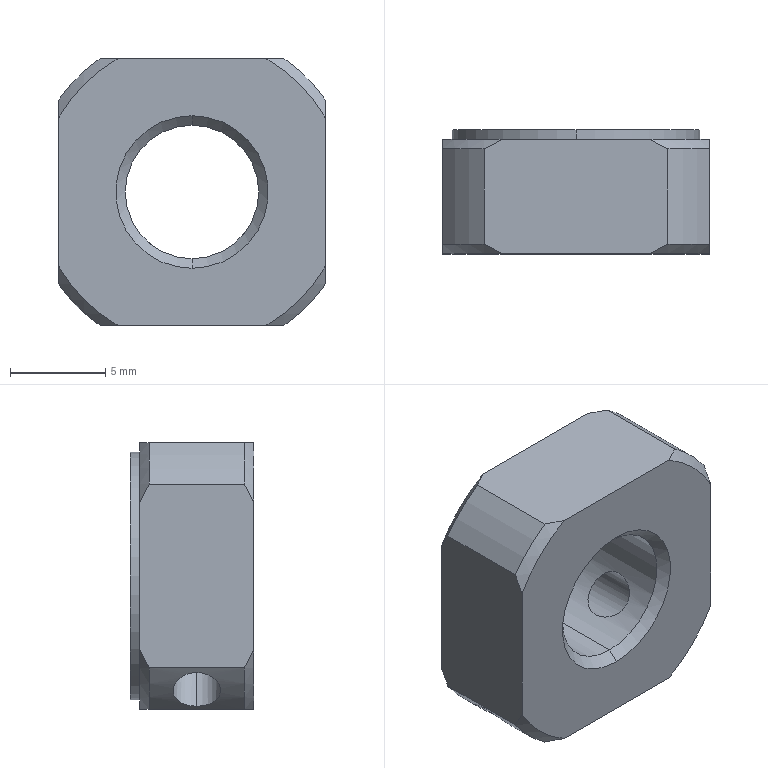Part | SolidWorks | features Chamfer 2, HoleWzd 2, ICE 2, CirPattern 1, Extrusion 1 | 1 solid | 31 faces | box 14 x 6.5 x 14 mm | volume 883.515 mm3 | cylinder 12 | cone 12 | plane 7 | commonest cylinder face diameters 2.5 x4 17 x4 7 x2 13 x2
STEP:
#1=CARTESIAN_POINT('',(-6.829,-3.,-5.061));
#2=VERTEX_POINT('',#1);
#3=CARTESIAN_POINT('',(-5.061,-3.,-6.829));
#4=VERTEX_POINT('',#3);
#5=CARTESIAN_POINT('',(-6.829,-3.,-5.061));
#6=CARTESIAN_POINT('',(-6.829,-3.163,-5.061));
#7=CARTESIAN_POINT('',(-6.809,-3.328,-5.088));
#8=CARTESIAN_POINT('',(-6.733,-3.629,-5.188));
#9=CARTESIAN_POINT('',(-6.676,-3.768,-5.262));
#10=CARTESIAN_POINT('',(-6.567,-3.941,-5.397));
#11=CARTESIAN_POINT('',(-6.526,-3.994,-5.447));
#12=CARTESIAN_POINT('',(-6.438,-4.084,-5.551));
#13=CARTESIAN_POINT('',(-6.391,-4.123,-5.605));
#14=CARTESIAN_POINT('',(-6.239,-4.217,-5.775));
#15=CARTESIAN_POINT('',(-6.128,-4.25,-5.893));
#16=CARTESIAN_POINT('',(-5.894,-4.25,-6.127));
#17=CARTESIAN_POINT('',(-5.776,-4.218,-6.238));
#18=CARTESIAN_POINT('',(-5.55,-4.092,-6.44));
#19=CARTESIAN_POINT('',(-5.443,-3.999,-6.53));
#20=CARTESIAN_POINT('',(-5.263,-3.769,-6.675));
#21=CARTESIAN_POINT('',(-5.189,-3.63,-6.733));
#22=CARTESIAN_POINT('',(-5.088,-3.33,-6.809));
#23=CARTESIAN_POINT('',(-5.061,-3.165,-6.829));
#24=CARTESIAN_POINT('',(-5.061,-3.,-6.829));
#25=B_SPLINE_CURVE_WITH_KNOTS('',3,(#5,#6,#7,#8,#9,#10,#11,#12,#13,#14,#15,#16,#17,#18,#19,#20,#21,#22,#23,#24),.UNSPECIFIED.,.F.,.F.,(4,2,2,2,2,2,2,2,2,4),(0.003913,0.004402,0.004891,0.005136,0.005381,0.00587,0.006359,0.006848,0.007337,0.007826),.UNSPECIFIED.);
#26=EDGE_CURVE('',#2,#4,#25,.T.);
#27=ORIENTED_EDGE('',*,*,#26,.F.);
#28=CARTESIAN_POINT('',(-3.196,-3.,-1.428));
#29=VERTEX_POINT('',#28);
#30=CARTESIAN_POINT('',(-0.8839,-3.,0.8839));
#31=DIRECTION('',(0.7071,0.,0.7071));
#32=VECTOR('',#31,1000.);
#33=LINE('',#30,#32);
#34=EDGE_CURVE('',#2,#29,#33,.T.);
#35=ORIENTED_EDGE('',*,*,#34,.T.);
#36=CARTESIAN_POINT('',(-1.428,-3.,-3.196));
#37=VERTEX_POINT('',#36);
#38=CARTESIAN_POINT('',(-1.428,-3.,-3.196));
#39=CARTESIAN_POINT('',(-1.428,-3.167,-3.196));
#40=CARTESIAN_POINT('',(-1.461,-3.33,-3.181));
#41=CARTESIAN_POINT('',(-1.581,-3.632,-3.123));
#42=CARTESIAN_POINT('',(-1.668,-3.77,-3.079));
#43=CARTESIAN_POINT('',(-1.872,-3.998,-2.96));
#44=CARTESIAN_POINT('',(-1.99,-4.091,-2.883));
#45=CARTESIAN_POINT('',(-2.232,-4.216,-2.7));
#46=CARTESIAN_POINT('',(-2.358,-4.25,-2.592));
#47=CARTESIAN_POINT('',(-2.533,-4.25,-2.417));
#48=CARTESIAN_POINT('',(-2.59,-4.242,-2.356));
#49=CARTESIAN_POINT('',(-2.695,-4.209,-2.234));
#50=CARTESIAN_POINT('',(-2.745,-4.186,-2.173));
#51=CARTESIAN_POINT('',(-2.884,-4.09,-1.989));
#52=CARTESIAN_POINT('',(-2.96,-3.998,-1.871));
#53=CARTESIAN_POINT('',(-3.05,-3.826,-1.718));
#54=CARTESIAN_POINT('',(-3.076,-3.763,-1.671));
#55=CARTESIAN_POINT('',(-3.12,-3.628,-1.587));
#56=CARTESIAN_POINT('',(-3.138,-3.555,-1.55));
#57=CARTESIAN_POINT('',(-3.181,-3.33,-1.461));
#58=CARTESIAN_POINT('',(-3.196,-3.164,-1.428));
#59=CARTESIAN_POINT('',(-3.196,-3.,-1.428));
#60=B_SPLINE_CURVE_WITH_KNOTS('',3,(#38,#39,#40,#41,#42,#43,#44,#45,#46,#47,#48,#49,#50,#51,#52,#53,#54,#55,#56,#57,#58,#59),.UNSPECIFIED.,.F.,.F.,(4,2,2,2,2,2,2,2,2,2,4),(0.,0.0004926,0.0009852,0.001478,0.00197,0.002217,0.002463,0.002956,0.003202,0.003448,0.003941),.UNSPECIFIED.);
#61=EDGE_CURVE('',#37,#29,#60,.T.);
#62=ORIENTED_EDGE('',*,*,#61,.F.);
#63=CARTESIAN_POINT('',(0.8839,-3.,-0.8839));
#64=DIRECTION('',(0.7071,0.,0.7071));
#65=VECTOR('',#64,1000.);
#66=LINE('',#63,#65);
#67=EDGE_CURVE('',#4,#37,#66,.T.);
#68=ORIENTED_EDGE('',*,*,#67,.F.);
#69=EDGE_LOOP('',(#27,#35,#62,#68));
#70=FACE_OUTER_BOUND('',#69,.T.);
#71=CARTESIAN_POINT('',(0.,-3.,0.));
#72=DIRECTION('',(0.7071,0.,0.7071));
#73=DIRECTION('',(0.7071,0.,-0.7071));
#74=AXIS2_PLACEMENT_3D('',#71,#72,#73);
#75=CYLINDRICAL_SURFACE('',#74,1.25);
#76=ADVANCED_FACE('',(#70),#75,.F.);
#77=CARTESIAN_POINT('',(0.,0.,-3.5));
#78=VERTEX_POINT('',#77);
#79=CARTESIAN_POINT('',(0.,0.,3.5));
#80=VERTEX_POINT('',#79);
#81=CARTESIAN_POINT('',(0.,0.,0.));
#82=DIRECTION('',(0.,1.,0.));
#83=DIRECTION('',(0.,0.,1.));
#84=AXIS2_PLACEMENT_3D('',#81,#82,#83);
#85=CIRCLE('',#84,3.5);
#86=EDGE_CURVE('',#78,#80,#85,.T.);
#87=ORIENTED_EDGE('',*,*,#86,.F.);
#88=CARTESIAN_POINT('',(0.,0.5,-4.));
#89=VERTEX_POINT('',#88);
#90=CARTESIAN_POINT('',(0.,0.,-3.5));
#91=DIRECTION('',(0.,0.7071,-0.7071));
#92=VECTOR('',#91,1000.);
#93=LINE('',#90,#92);
#94=EDGE_CURVE('',#78,#89,#93,.T.);
#95=ORIENTED_EDGE('',*,*,#94,.T.);
#96=CARTESIAN_POINT('',(0.,0.5,4.));
#97=VERTEX_POINT('',#96);
#98=CARTESIAN_POINT('',(0.,0.5,0.));
#99=DIRECTION('',(0.,-1.,0.));
#100=DIRECTION('',(0.,0.,1.));
#101=AXIS2_PLACEMENT_3D('',#98,#99,#100);
#102=CIRCLE('',#101,4.);
#103=EDGE_CURVE('',#97,#89,#102,.T.);
#104=ORIENTED_EDGE('',*,*,#103,.F.);
#105=CARTESIAN_POINT('',(0.,0.,3.5));
#106=DIRECTION('',(0.,0.7071,0.7071));
#107=VECTOR('',#106,1000.);
#108=LINE('',#105,#107);
#109=EDGE_CURVE('',#80,#97,#108,.T.);
#110=ORIENTED_EDGE('',*,*,#109,.F.);
#111=EDGE_LOOP('',(#87,#95,#104,#110));
#112=FACE_OUTER_BOUND('',#111,.T.);
#113=CARTESIAN_POINT('',(0.,0.,0.));
#114=DIRECTION('',(0.,1.,0.));
#115=DIRECTION('',(0.,0.,1.));
#116=AXIS2_PLACEMENT_3D('',#113,#114,#115);
#117=CONICAL_SURFACE('',#116,3.5,0.7854);
#118=ADVANCED_FACE('',(#112),#117,.F.);
#119=CARTESIAN_POINT('',(0.,-5.5,3.5));
#120=VERTEX_POINT('',#119);
#121=CARTESIAN_POINT('',(0.,-5.5,-3.5));
#122=VERTEX_POINT('',#121);
#123=CARTESIAN_POINT('',(0.,-5.5,0.));
#124=DIRECTION('',(0.,-1.,0.));
#125=DIRECTION('',(0.,0.,-1.));
#126=AXIS2_PLACEMENT_3D('',#123,#124,#125);
#127=CIRCLE('',#126,3.5);
#128=EDGE_CURVE('',#120,#122,#127,.T.);
#129=ORIENTED_EDGE('',*,*,#128,.F.);
#130=CARTESIAN_POINT('',(0.,-6.,4.));
#131=VERTEX_POINT('',#130);
#132=CARTESIAN_POINT('',(0.,-5.5,3.5));
#133=DIRECTION('',(0.,-0.7071,0.7071));
#134=VECTOR('',#133,1000.);
#135=LINE('',#132,#134);
#136=EDGE_CURVE('',#120,#131,#135,.T.);
#137=ORIENTED_EDGE('',*,*,#136,.T.);
#138=CARTESIAN_POINT('',(0.,-6.,-4.));
#139=VERTEX_POINT('',#138);
#140=CARTESIAN_POINT('',(0.,-6.,0.));
#141=DIRECTION('',(0.,1.,0.));
#142=DIRECTION('',(0.,0.,-1.));
#143=AXIS2_PLACEMENT_3D('',#140,#141,#142);
#144=CIRCLE('',#143,4.);
#145=EDGE_CURVE('',#139,#131,#144,.T.);
#146=ORIENTED_EDGE('',*,*,#145,.F.);
#147=CARTESIAN_POINT('',(0.,-5.5,-3.5));
#148=DIRECTION('',(0.,-0.7071,-0.7071));
#149=VECTOR('',#148,1000.);
#150=LINE('',#147,#149);
#151=EDGE_CURVE('',#122,#139,#150,.T.);
#152=ORIENTED_EDGE('',*,*,#151,.F.);
#153=EDGE_LOOP('',(#129,#137,#146,#152));
#154=FACE_OUTER_BOUND('',#153,.T.);
#155=CARTESIAN_POINT('',(0.,-5.5,0.));
#156=DIRECTION('',(0.,-1.,0.));
#157=DIRECTION('',(0.,0.,-1.));
#158=AXIS2_PLACEMENT_3D('',#155,#156,#157);
#159=CONICAL_SURFACE('',#158,3.5,0.7854);
#160=ADVANCED_FACE('',(#154),#159,.F.);
#161=CARTESIAN_POINT('',(5.061,-3.,-6.829));
#162=VERTEX_POINT('',#161);
#163=CARTESIAN_POINT('',(6.829,-3.,-5.061));
#164=VERTEX_POINT('',#163);
#165=CARTESIAN_POINT('',(5.061,-3.,-6.829));
#166=CARTESIAN_POINT('',(5.061,-3.163,-6.829));
#167=CARTESIAN_POINT('',(5.088,-3.328,-6.809));
#168=CARTESIAN_POINT('',(5.188,-3.629,-6.733));
#169=CARTESIAN_POINT('',(5.262,-3.768,-6.676));
#170=CARTESIAN_POINT('',(5.397,-3.941,-6.567));
#171=CARTESIAN_POINT('',(5.447,-3.994,-6.526));
#172=CARTESIAN_POINT('',(5.551,-4.084,-6.438));
#173=CARTESIAN_POINT('',(5.605,-4.123,-6.391));
#174=CARTESIAN_POINT('',(5.775,-4.217,-6.239));
#175=CARTESIAN_POINT('',(5.893,-4.25,-6.128));
#176=CARTESIAN_POINT('',(6.127,-4.25,-5.894));
#177=CARTESIAN_POINT('',(6.238,-4.218,-5.776));
#178=CARTESIAN_POINT('',(6.44,-4.092,-5.55));
#179=CARTESIAN_POINT('',(6.53,-3.999,-5.443));
#180=CARTESIAN_POINT('',(6.675,-3.769,-5.263));
#181=CARTESIAN_POINT('',(6.733,-3.63,-5.189));
#182=CARTESIAN_POINT('',(6.809,-3.33,-5.088));
#183=CARTESIAN_POINT('',(6.829,-3.165,-5.061));
#184=CARTESIAN_POINT('',(6.829,-3.,-5.061));
#185=B_SPLINE_CURVE_WITH_KNOTS('',3,(#165,#166,#167,#168,#169,#170,#171,#172,#173,#174,#175,#176,#177,#178,#179,#180,#181,#182,#183,#184),.UNSPECIFIED.,.F.,.F.,(4,2,2,2,2,2,2,2,2,4),(0.003913,0.004402,0.004891,0.005136,0.005381,0.00587,0.006359,0.006848,0.007337,0.007826),.UNSPECIFIED.);
#186=EDGE_CURVE('',#162,#164,#185,.T.);
#187=ORIENTED_EDGE('',*,*,#186,.F.);
#188=CARTESIAN_POINT('',(1.428,-3.,-3.196));
#189=VERTEX_POINT('',#188);
#190=CARTESIAN_POINT('',(-0.8839,-3.,-0.8839));
#191=DIRECTION('',(-0.7071,0.,0.7071));
#192=VECTOR('',#191,1000.);
#193=LINE('',#190,#192);
#194=EDGE_CURVE('',#162,#189,#193,.T.);
#195=ORIENTED_EDGE('',*,*,#194,.T.);
#196=CARTESIAN_POINT('',(3.196,-3.,-1.428));
#197=VERTEX_POINT('',#196);
#198=CARTESIAN_POINT('',(3.196,-3.,-1.428));
#199=CARTESIAN_POINT('',(3.196,-3.167,-1.428));
#200=CARTESIAN_POINT('',(3.181,-3.33,-1.461));
#201=CARTESIAN_POINT('',(3.123,-3.632,-1.581));
#202=CARTESIAN_POINT('',(3.079,-3.77,-1.668));
#203=CARTESIAN_POINT('',(2.96,-3.998,-1.872));
#204=CARTESIAN_POINT('',(2.883,-4.091,-1.99));
#205=CARTESIAN_POINT('',(2.7,-4.216,-2.232));
#206=CARTESIAN_POINT('',(2.592,-4.25,-2.358));
#207=CARTESIAN_POINT('',(2.417,-4.25,-2.533));
#208=CARTESIAN_POINT('',(2.356,-4.242,-2.59));
#209=CARTESIAN_POINT('',(2.234,-4.209,-2.695));
#210=CARTESIAN_POINT('',(2.173,-4.186,-2.745));
#211=CARTESIAN_POINT('',(1.989,-4.09,-2.884));
#212=CARTESIAN_POINT('',(1.871,-3.998,-2.96));
#213=CARTESIAN_POINT('',(1.718,-3.826,-3.05));
#214=CARTESIAN_POINT('',(1.671,-3.763,-3.076));
#215=CARTESIAN_POINT('',(1.587,-3.628,-3.12));
#216=CARTESIAN_POINT('',(1.55,-3.555,-3.138));
#217=CARTESIAN_POINT('',(1.461,-3.33,-3.181));
#218=CARTESIAN_POINT('',(1.428,-3.164,-3.196));
#219=CARTESIAN_POINT('',(1.428,-3.,-3.196));
#220=B_SPLINE_CURVE_WITH_KNOTS('',3,(#198,#199,#200,#201,#202,#203,#204,#205,#206,#207,#208,#209,#210,#211,#212,#213,#214,#215,#216,#217,#218,#219),.UNSPECIFIED.,.F.,.F.,(4,2,2,2,2,2,2,2,2,2,4),(0.,0.0004926,0.0009852,0.001478,0.00197,0.002217,0.002463,0.002956,0.003202,0.003448,0.003941),.UNSPECIFIED.);
#221=EDGE_CURVE('',#197,#189,#220,.T.);
#222=ORIENTED_EDGE('',*,*,#221,.F.);
#223=CARTESIAN_POINT('',(0.8839,-3.,0.8839));
#224=DIRECTION('',(-0.7071,0.,0.7071));
#225=VECTOR('',#224,1000.);
#226=LINE('',#223,#225);
#227=EDGE_CURVE('',#164,#197,#226,.T.);
#228=ORIENTED_EDGE('',*,*,#227,.F.);
#229=EDGE_LOOP('',(#187,#195,#222,#228));
#230=FACE_OUTER_BOUND('',#229,.T.);
#231=CARTESIAN_POINT('',(0.,-3.,0.));
#232=DIRECTION('',(-0.7071,0.,0.7071));
#233=DIRECTION('',(0.7071,0.,0.7071));
#234=AXIS2_PLACEMENT_3D('',#231,#232,#233);
#235=CYLINDRICAL_SURFACE('',#234,1.25);
#236=ADVANCED_FACE('',(#230),#235,.F.);
#237=ORIENTED_EDGE('',*,*,#61,.T.);
#238=CARTESIAN_POINT('',(-3.196,-3.,-1.428));
#239=CARTESIAN_POINT('',(-3.196,-2.836,-1.428));
#240=CARTESIAN_POINT('',(-3.181,-2.67,-1.461));
#241=CARTESIAN_POINT('',(-3.124,-2.369,-1.58));
#242=CARTESIAN_POINT('',(-3.08,-2.232,-1.667));
#243=CARTESIAN_POINT('',(-2.959,-2.,-1.873));
#244=CARTESIAN_POINT('',(-2.883,-1.909,-1.99));
#245=CARTESIAN_POINT('',(-2.745,-1.814,-2.173));
#246=CARTESIAN_POINT('',(-2.695,-1.791,-2.234));
#247=CARTESIAN_POINT('',(-2.59,-1.758,-2.356));
#248=CARTESIAN_POINT('',(-2.533,-1.75,-2.417));
#249=CARTESIAN_POINT('',(-2.358,-1.75,-2.592));
#250=CARTESIAN_POINT('',(-2.232,-1.784,-2.7));
#251=CARTESIAN_POINT('',(-1.99,-1.909,-2.883));
#252=CARTESIAN_POINT('',(-1.871,-2.002,-2.96));
#253=CARTESIAN_POINT('',(-1.667,-2.231,-3.08));
#254=CARTESIAN_POINT('',(-1.581,-2.368,-3.123));
#255=CARTESIAN_POINT('',(-1.46,-2.671,-3.181));
#256=CARTESIAN_POINT('',(-1.428,-2.833,-3.196));
#257=CARTESIAN_POINT('',(-1.428,-3.,-3.196));
#258=B_SPLINE_CURVE_WITH_KNOTS('',3,(#238,#239,#240,#241,#242,#243,#244,#245,#246,#247,#248,#249,#250,#251,#252,#253,#254,#255,#256,#257),.UNSPECIFIED.,.F.,.F.,(4,2,2,2,2,2,2,2,2,4),(0.003941,0.004433,0.004926,0.005418,0.005664,0.005911,0.006403,0.006896,0.007388,0.007881),.UNSPECIFIED.);
#259=EDGE_CURVE('',#29,#37,#258,.T.);
#260=ORIENTED_EDGE('',*,*,#259,.T.);
#261=EDGE_LOOP('',(#237,#260));
#262=FACE_BOUND('',#261,.T.);
#263=ORIENTED_EDGE('',*,*,#128,.T.);
#264=CARTESIAN_POINT('',(0.,0.5,-3.5));
#265=DIRECTION('',(0.,1.,0.));
#266=VECTOR('',#265,1000.);
#267=LINE('',#264,#266);
#268=EDGE_CURVE('',#122,#78,#267,.T.);
#269=ORIENTED_EDGE('',*,*,#268,.T.);
#270=ORIENTED_EDGE('',*,*,#86,.T.);
#271=CARTESIAN_POINT('',(0.,0.5,3.5));
#272=DIRECTION('',(0.,1.,0.));
#273=VECTOR('',#272,1000.);
#274=LINE('',#271,#273);
#275=EDGE_CURVE('',#120,#80,#274,.T.);
#276=ORIENTED_EDGE('',*,*,#275,.F.);
#277=EDGE_LOOP('',(#263,#269,#270,#276));
#278=FACE_OUTER_BOUND('',#277,.T.);
#279=CARTESIAN_POINT('',(0.,0.5,0.));
#280=DIRECTION('',(0.,1.,0.));
#281=DIRECTION('',(0.,0.,1.));
#282=AXIS2_PLACEMENT_3D('',#279,#280,#281);
#283=CYLINDRICAL_SURFACE('',#282,3.5);
#284=ADVANCED_FACE('',(#262,#278),#283,.F.);
#285=CARTESIAN_POINT('',(0.,0.5,6.5));
#286=VERTEX_POINT('',#285);
#287=CARTESIAN_POINT('',(0.,0.5,-6.5));
#288=VERTEX_POINT('',#287);
#289=CARTESIAN_POINT('',(0.,0.5,0.));
#290=DIRECTION('',(0.,1.,0.));
#291=DIRECTION('',(0.,0.,1.));
#292=AXIS2_PLACEMENT_3D('',#289,#290,#291);
#293=CIRCLE('',#292,6.5);
#294=EDGE_CURVE('',#286,#288,#293,.T.);
#295=ORIENTED_EDGE('',*,*,#294,.F.);
#296=CARTESIAN_POINT('',(0.,0.,6.5));
#297=VERTEX_POINT('',#296);
#298=CARTESIAN_POINT('',(0.,0.5,6.5));
#299=DIRECTION('',(0.,-1.,0.));
#300=VECTOR('',#299,1000.);
#301=LINE('',#298,#300);
#302=EDGE_CURVE('',#286,#297,#301,.T.);
#303=ORIENTED_EDGE('',*,*,#302,.T.);
#304=CARTESIAN_POINT('',(0.,0.,-6.5));
#305=VERTEX_POINT('',#304);
#306=CARTESIAN_POINT('',(0.,0.,0.));
#307=DIRECTION('',(0.,-1.,0.));
#308=DIRECTION('',(0.,0.,-1.));
#309=AXIS2_PLACEMENT_3D('',#306,#307,#308);
#310=CIRCLE('',#309,6.5);
#311=EDGE_CURVE('',#305,#297,#310,.T.);
#312=ORIENTED_EDGE('',*,*,#311,.F.);
#313=CARTESIAN_POINT('',(0.,0.5,-6.5));
#314=DIRECTION('',(0.,-1.,0.));
#315=VECTOR('',#314,1000.);
#316=LINE('',#313,#315);
#317=EDGE_CURVE('',#288,#305,#316,.T.);
#318=ORIENTED_EDGE('',*,*,#317,.F.);
#319=EDGE_LOOP('',(#295,#303,#312,#318));
#320=FACE_OUTER_BOUND('',#319,.T.);
#321=CARTESIAN_POINT('',(0.,0.5,0.));
#322=DIRECTION('',(0.,-1.,0.));
#323=DIRECTION('',(0.,0.,-1.));
#324=AXIS2_PLACEMENT_3D('',#321,#322,#323);
#325=CYLINDRICAL_SURFACE('',#324,6.5);
#326=ADVANCED_FACE('',(#320),#325,.T.);
#327=CARTESIAN_POINT('',(-7.,-5.5,4.822));
#328=VERTEX_POINT('',#327);
#329=CARTESIAN_POINT('',(-4.822,-5.5,7.));
#330=VERTEX_POINT('',#329);
#331=CARTESIAN_POINT('',(0.,-5.5,0.));
#332=DIRECTION('',(0.,1.,0.));
#333=DIRECTION('',(0.,0.,-1.));
#334=AXIS2_PLACEMENT_3D('',#331,#332,#333);
#335=CIRCLE('',#334,8.5);
#336=EDGE_CURVE('',#328,#330,#335,.T.);
#337=ORIENTED_EDGE('',*,*,#336,.T.);
#338=CARTESIAN_POINT('',(-4.822,-0.5,7.));
#339=VERTEX_POINT('',#338);
#340=CARTESIAN_POINT('',(-4.822,-6.,7.));
#341=DIRECTION('',(0.,1.,0.));
#342=VECTOR('',#341,1000.);
#343=LINE('',#340,#342);
#344=EDGE_CURVE('',#330,#339,#343,.T.);
#345=ORIENTED_EDGE('',*,*,#344,.T.);
#346=CARTESIAN_POINT('',(-7.,-0.5,4.822));
#347=VERTEX_POINT('',#346);
#348=CARTESIAN_POINT('',(0.,-0.5,0.));
#349=DIRECTION('',(0.,-1.,0.));
#350=DIRECTION('',(0.,0.,-1.));
#351=AXIS2_PLACEMENT_3D('',#348,#349,#350);
#352=CIRCLE('',#351,8.5);
#353=EDGE_CURVE('',#339,#347,#352,.T.);
#354=ORIENTED_EDGE('',*,*,#353,.T.);
#355=CARTESIAN_POINT('',(-7.,-6.,4.822));
#356=DIRECTION('',(0.,-1.,0.));
#357=VECTOR('',#356,1000.);
#358=LINE('',#355,#357);
#359=EDGE_CURVE('',#347,#328,#358,.T.);
#360=ORIENTED_EDGE('',*,*,#359,.T.);
#361=EDGE_LOOP('',(#337,#345,#354,#360));
#362=FACE_OUTER_BOUND('',#361,.T.);
#363=CARTESIAN_POINT('',(0.,-6.,0.));
#364=DIRECTION('',(0.,1.,0.));
#365=DIRECTION('',(0.,0.,1.));
#366=AXIS2_PLACEMENT_3D('',#363,#364,#365);
#367=CYLINDRICAL_SURFACE('',#366,8.5);
#368=ADVANCED_FACE('',(#362),#367,.T.);
#369=CARTESIAN_POINT('',(-3.873,-6.,7.));
#370=VERTEX_POINT('',#369);
#371=CARTESIAN_POINT('',(-4.822,-5.5,7.));
#372=CARTESIAN_POINT('',(-4.511,-5.676,7.));
#373=CARTESIAN_POINT('',(-4.195,-5.844,7.));
#374=CARTESIAN_POINT('',(-3.873,-6.,7.));
#375=B_SPLINE_CURVE_WITH_KNOTS('',3,(#371,#372,#373,#374),.UNSPECIFIED.,.F.,.F.,(4,4),(0.00829,0.009369),.UNSPECIFIED.);
#376=EDGE_CURVE('',#330,#370,#375,.T.);
#377=ORIENTED_EDGE('',*,*,#376,.F.);
#378=ORIENTED_EDGE('',*,*,#336,.F.);
#379=CARTESIAN_POINT('',(-7.,-6.,3.873));
#380=VERTEX_POINT('',#379);
#381=CARTESIAN_POINT('',(-7.,-6.,3.873));
#382=CARTESIAN_POINT('',(-7.,-5.844,4.195));
#383=CARTESIAN_POINT('',(-7.,-5.676,4.511));
#384=CARTESIAN_POINT('',(-7.,-5.5,4.822));
#385=B_SPLINE_CURVE_WITH_KNOTS('',3,(#381,#382,#383,#384),.UNSPECIFIED.,.F.,.F.,(4,4),(0.02473,0.02581),.UNSPECIFIED.);
#386=EDGE_CURVE('',#380,#328,#385,.T.);
#387=ORIENTED_EDGE('',*,*,#386,.F.);
#388=CARTESIAN_POINT('',(0.,-6.,0.));
#389=DIRECTION('',(0.,-1.,0.));
#390=DIRECTION('',(0.,0.,-1.));
#391=AXIS2_PLACEMENT_3D('',#388,#389,#390);
#392=CIRCLE('',#391,8.);
#393=EDGE_CURVE('',#370,#380,#392,.T.);
#394=ORIENTED_EDGE('',*,*,#393,.F.);
#395=EDGE_LOOP('',(#377,#378,#387,#394));
#396=FACE_OUTER_BOUND('',#395,.T.);
#397=CARTESIAN_POINT('',(0.,-6.,0.));
#398=DIRECTION('',(0.,1.,0.));
#399=DIRECTION('',(0.,0.,1.));
#400=AXIS2_PLACEMENT_3D('',#397,#398,#399);
#401=CONICAL_SURFACE('',#400,8.,0.7854);
#402=ADVANCED_FACE('',(#396),#401,.T.);
#403=CARTESIAN_POINT('',(4.822,-0.5,7.));
#404=VERTEX_POINT('',#403);
#405=CARTESIAN_POINT('',(3.873,0.,7.));
#406=VERTEX_POINT('',#405);
#407=CARTESIAN_POINT('',(4.822,-0.5,7.));
#408=CARTESIAN_POINT('',(4.511,-0.3235,7.));
#409=CARTESIAN_POINT('',(4.195,-0.1559,7.));
#410=CARTESIAN_POINT('',(3.873,0.,7.));
#411=B_SPLINE_CURVE_WITH_KNOTS('',3,(#407,#408,#409,#410),.UNSPECIFIED.,.F.,.F.,(4,4),(0.007915,0.008995),.UNSPECIFIED.);
#412=EDGE_CURVE('',#404,#406,#411,.T.);
#413=ORIENTED_EDGE('',*,*,#412,.F.);
#414=CARTESIAN_POINT('',(7.,-0.5,4.822));
#415=VERTEX_POINT('',#414);
#416=CARTESIAN_POINT('',(0.,-0.5,0.));
#417=DIRECTION('',(0.,-1.,0.));
#418=DIRECTION('',(0.,0.,-1.));
#419=AXIS2_PLACEMENT_3D('',#416,#417,#418);
#420=CIRCLE('',#419,8.5);
#421=EDGE_CURVE('',#415,#404,#420,.T.);
#422=ORIENTED_EDGE('',*,*,#421,.F.);
#423=CARTESIAN_POINT('',(7.,0.,3.873));
#424=VERTEX_POINT('',#423);
#425=CARTESIAN_POINT('',(7.,0.,3.873));
#426=CARTESIAN_POINT('',(7.,-0.1561,4.196));
#427=CARTESIAN_POINT('',(7.,-0.3238,4.511));
#428=CARTESIAN_POINT('',(7.,-0.5,4.822));
#429=B_SPLINE_CURVE_WITH_KNOTS('',3,(#425,#426,#427,#428),.UNSPECIFIED.,.F.,.F.,(4,4),(0.02391,0.025),.UNSPECIFIED.);
#430=EDGE_CURVE('',#424,#415,#429,.T.);
#431=ORIENTED_EDGE('',*,*,#430,.F.);
#432=CARTESIAN_POINT('',(0.,0.,0.));
#433=DIRECTION('',(0.,1.,0.));
#434=DIRECTION('',(0.,0.,-1.));
#435=AXIS2_PLACEMENT_3D('',#432,#433,#434);
#436=CIRCLE('',#435,8.);
#437=EDGE_CURVE('',#406,#424,#436,.T.);
#438=ORIENTED_EDGE('',*,*,#437,.F.);
#439=EDGE_LOOP('',(#413,#422,#431,#438));
#440=FACE_OUTER_BOUND('',#439,.T.);
#441=CARTESIAN_POINT('',(0.,-0.5,0.));
#442=DIRECTION('',(0.,-1.,0.));
#443=DIRECTION('',(0.,0.,-1.));
#444=AXIS2_PLACEMENT_3D('',#441,#442,#443);
#445=CONICAL_SURFACE('',#444,8.5,0.7854);
#446=ADVANCED_FACE('',(#440),#445,.T.);
#447=ORIENTED_EDGE('',*,*,#421,.T.);
#448=CARTESIAN_POINT('',(4.822,-5.5,7.));
#449=VERTEX_POINT('',#448);
#450=CARTESIAN_POINT('',(4.822,-6.,7.));
#451=DIRECTION('',(0.,-1.,0.));
#452=VECTOR('',#451,1000.);
#453=LINE('',#450,#452);
#454=EDGE_CURVE('',#404,#449,#453,.T.);
#455=ORIENTED_EDGE('',*,*,#454,.T.);
#456=CARTESIAN_POINT('',(7.,-5.5,4.822));
#457=VERTEX_POINT('',#456);
#458=CARTESIAN_POINT('',(0.,-5.5,0.));
#459=DIRECTION('',(0.,1.,0.));
#460=DIRECTION('',(0.,0.,-1.));
#461=AXIS2_PLACEMENT_3D('',#458,#459,#460);
#462=CIRCLE('',#461,8.5);
#463=EDGE_CURVE('',#449,#457,#462,.T.);
#464=ORIENTED_EDGE('',*,*,#463,.T.);
#465=CARTESIAN_POINT('',(7.,-6.,4.822));
#466=DIRECTION('',(0.,1.,0.));
#467=VECTOR('',#466,1000.);
#468=LINE('',#465,#467);
#469=EDGE_CURVE('',#457,#415,#468,.T.);
#470=ORIENTED_EDGE('',*,*,#469,.T.);
#471=EDGE_LOOP('',(#447,#455,#464,#470));
#472=FACE_OUTER_BOUND('',#471,.T.);
#473=CARTESIAN_POINT('',(0.,-6.,0.));
#474=DIRECTION('',(0.,1.,0.));
#475=DIRECTION('',(0.,0.,1.));
#476=AXIS2_PLACEMENT_3D('',#473,#474,#475);
#477=CYLINDRICAL_SURFACE('',#476,8.5);
#478=ADVANCED_FACE('',(#472),#477,.T.);
#479=CARTESIAN_POINT('',(3.873,-6.,7.));
#480=VERTEX_POINT('',#479);
#481=CARTESIAN_POINT('',(3.873,-6.,7.));
#482=CARTESIAN_POINT('',(4.196,-5.844,7.));
#483=CARTESIAN_POINT('',(4.512,-5.676,7.));
#484=CARTESIAN_POINT('',(4.822,-5.5,7.));
#485=B_SPLINE_CURVE_WITH_KNOTS('',3,(#481,#482,#483,#484),.UNSPECIFIED.,.F.,.F.,(4,4),(0.01741,0.01848),.UNSPECIFIED.);
#486=EDGE_CURVE('',#480,#449,#485,.T.);
#487=ORIENTED_EDGE('',*,*,#486,.F.);
#488=CARTESIAN_POINT('',(7.,-6.,3.873));
#489=VERTEX_POINT('',#488);
#490=CARTESIAN_POINT('',(0.,-6.,0.));
#491=DIRECTION('',(0.,-1.,0.));
#492=DIRECTION('',(0.,0.,-1.));
#493=AXIS2_PLACEMENT_3D('',#490,#491,#492);
#494=CIRCLE('',#493,8.);
#495=EDGE_CURVE('',#489,#480,#494,.T.);
#496=ORIENTED_EDGE('',*,*,#495,.F.);
#497=CARTESIAN_POINT('',(7.,-5.5,4.822));
#498=CARTESIAN_POINT('',(7.,-5.677,4.51));
#499=CARTESIAN_POINT('',(7.,-5.844,4.194));
#500=CARTESIAN_POINT('',(7.,-6.,3.873));
#501=B_SPLINE_CURVE_WITH_KNOTS('',3,(#497,#498,#499,#500),.UNSPECIFIED.,.F.,.F.,(4,4),(0.01486,0.01593),.UNSPECIFIED.);
#502=EDGE_CURVE('',#457,#489,#501,.T.);
#503=ORIENTED_EDGE('',*,*,#502,.F.);
#504=ORIENTED_EDGE('',*,*,#463,.F.);
#505=EDGE_LOOP('',(#487,#496,#503,#504));
#506=FACE_OUTER_BOUND('',#505,.T.);
#507=CARTESIAN_POINT('',(0.,-6.,0.));
#508=DIRECTION('',(0.,1.,0.));
#509=DIRECTION('',(0.,0.,1.));
#510=AXIS2_PLACEMENT_3D('',#507,#508,#509);
#511=CONICAL_SURFACE('',#510,8.,0.7854);
#512=ADVANCED_FACE('',(#506),#511,.T.);
#513=CARTESIAN_POINT('',(7.,-0.5,-4.822));
#514=VERTEX_POINT('',#513);
#515=CARTESIAN_POINT('',(7.,0.,-3.873));
#516=VERTEX_POINT('',#515);
#517=CARTESIAN_POINT('',(7.,-0.5,-4.822));
#518=CARTESIAN_POINT('',(7.,-0.3232,-4.51));
#519=CARTESIAN_POINT('',(7.,-0.1556,-4.194));
#520=CARTESIAN_POINT('',(7.,0.,-3.873));
#521=B_SPLINE_CURVE_WITH_KNOTS('',3,(#517,#518,#519,#520),.UNSPECIFIED.,.F.,.F.,(4,4),(0.01477,0.01584),.UNSPECIFIED.);
#522=EDGE_CURVE('',#514,#516,#521,.T.);
#523=ORIENTED_EDGE('',*,*,#522,.F.);
#524=CARTESIAN_POINT('',(4.822,-0.5,-7.));
#525=VERTEX_POINT('',#524);
#526=CARTESIAN_POINT('',(0.,-0.5,0.));
#527=DIRECTION('',(0.,-1.,0.));
#528=DIRECTION('',(0.,0.,-1.));
#529=AXIS2_PLACEMENT_3D('',#526,#527,#528);
#530=CIRCLE('',#529,8.5);
#531=EDGE_CURVE('',#525,#514,#530,.T.);
#532=ORIENTED_EDGE('',*,*,#531,.F.);
#533=CARTESIAN_POINT('',(3.873,0.,-7.));
#534=VERTEX_POINT('',#533);
#535=CARTESIAN_POINT('',(3.873,0.,-7.));
#536=CARTESIAN_POINT('',(4.196,-0.1565,-7.));
#537=CARTESIAN_POINT('',(4.512,-0.3242,-7.));
#538=CARTESIAN_POINT('',(4.822,-0.5,-7.));
#539=B_SPLINE_CURVE_WITH_KNOTS('',3,(#535,#536,#537,#538),.UNSPECIFIED.,.F.,.F.,(4,4),(0.01686,0.01793),.UNSPECIFIED.);
#540=EDGE_CURVE('',#534,#525,#539,.T.);
#541=ORIENTED_EDGE('',*,*,#540,.F.);
#542=CARTESIAN_POINT('',(0.,0.,0.));
#543=DIRECTION('',(0.,1.,0.));
#544=DIRECTION('',(0.,0.,-1.));
#545=AXIS2_PLACEMENT_3D('',#542,#543,#544);
#546=CIRCLE('',#545,8.);
#547=EDGE_CURVE('',#516,#534,#546,.T.);
#548=ORIENTED_EDGE('',*,*,#547,.F.);
#549=EDGE_LOOP('',(#523,#532,#541,#548));
#550=FACE_OUTER_BOUND('',#549,.T.);
#551=CARTESIAN_POINT('',(0.,-0.5,0.));
#552=DIRECTION('',(0.,-1.,0.));
#553=DIRECTION('',(0.,0.,-1.));
#554=AXIS2_PLACEMENT_3D('',#551,#552,#553);
#555=CONICAL_SURFACE('',#554,8.5,0.7854);
#556=ADVANCED_FACE('',(#550),#555,.T.);
#557=CARTESIAN_POINT('',(6.829,-3.,-5.061));
#558=CARTESIAN_POINT('',(6.829,-2.835,-5.061));
#559=CARTESIAN_POINT('',(6.809,-2.672,-5.088));
#560=CARTESIAN_POINT('',(6.733,-2.37,-5.189));
#561=CARTESIAN_POINT('',(6.676,-2.231,-5.263));
#562=CARTESIAN_POINT('',(6.53,-2.001,-5.443));
#563=CARTESIAN_POINT('',(6.44,-1.908,-5.55));
#564=CARTESIAN_POINT('',(6.239,-1.783,-5.775));
#565=CARTESIAN_POINT('',(6.126,-1.75,-5.895));
#566=CARTESIAN_POINT('',(5.953,-1.75,-6.068));
#567=CARTESIAN_POINT('',(5.893,-1.758,-6.126));
#568=CARTESIAN_POINT('',(5.777,-1.79,-6.236));
#569=CARTESIAN_POINT('',(5.719,-1.814,-6.289));
#570=CARTESIAN_POINT('',(5.55,-1.908,-6.44));
#571=CARTESIAN_POINT('',(5.444,-2.,-6.529));
#572=CARTESIAN_POINT('',(5.262,-2.233,-6.677));
#573=CARTESIAN_POINT('',(5.189,-2.37,-6.733));
#574=CARTESIAN_POINT('',(5.113,-2.597,-6.79));
#575=CARTESIAN_POINT('',(5.094,-2.675,-6.805));
#576=CARTESIAN_POINT('',(5.068,-2.835,-6.824));
#577=CARTESIAN_POINT('',(5.061,-2.918,-6.829));
#578=CARTESIAN_POINT('',(5.061,-3.,-6.829));
#579=B_SPLINE_CURVE_WITH_KNOTS('',3,(#557,#558,#559,#560,#561,#562,#563,#564,#565,#566,#567,#568,#569,#570,#571,#572,#573,#574,#575,#576,#577,#578),.UNSPECIFIED.,.F.,.F.,(4,2,2,2,2,2,2,2,2,2,4),(0.,0.0004892,0.0009783,0.001468,0.001957,0.002201,0.002446,0.002935,0.003424,0.003669,0.003913),.UNSPECIFIED.);
#580=EDGE_CURVE('',#164,#162,#579,.T.);
#581=ORIENTED_EDGE('',*,*,#580,.T.);
#582=ORIENTED_EDGE('',*,*,#186,.T.);
#583=EDGE_LOOP('',(#581,#582));
#584=FACE_BOUND('',#583,.T.);
#585=ORIENTED_EDGE('',*,*,#531,.T.);
#586=CARTESIAN_POINT('',(7.,-5.5,-4.822));
#587=VERTEX_POINT('',#586);
#588=CARTESIAN_POINT('',(7.,-6.,-4.822));
#589=DIRECTION('',(0.,-1.,0.));
#590=VECTOR('',#589,1000.);
#591=LINE('',#588,#590);
#592=EDGE_CURVE('',#514,#587,#591,.T.);
#593=ORIENTED_EDGE('',*,*,#592,.T.);
#594=CARTESIAN_POINT('',(4.822,-5.5,-7.));
#595=VERTEX_POINT('',#594);
#596=CARTESIAN_POINT('',(0.,-5.5,0.));
#597=DIRECTION('',(0.,1.,0.));
#598=DIRECTION('',(0.,0.,-1.));
#599=AXIS2_PLACEMENT_3D('',#596,#597,#598);
#600=CIRCLE('',#599,8.5);
#601=EDGE_CURVE('',#587,#595,#600,.T.);
#602=ORIENTED_EDGE('',*,*,#601,.T.);
#603=CARTESIAN_POINT('',(4.822,-6.,-7.));
#604=DIRECTION('',(0.,1.,0.));
#605=VECTOR('',#604,1000.);
#606=LINE('',#603,#605);
#607=EDGE_CURVE('',#595,#525,#606,.T.);
#608=ORIENTED_EDGE('',*,*,#607,.T.);
#609=EDGE_LOOP('',(#585,#593,#602,#608));
#610=FACE_OUTER_BOUND('',#609,.T.);
#611=CARTESIAN_POINT('',(0.,-6.,0.));
#612=DIRECTION('',(0.,1.,0.));
#613=DIRECTION('',(0.,0.,1.));
#614=AXIS2_PLACEMENT_3D('',#611,#612,#613);
#615=CYLINDRICAL_SURFACE('',#614,8.5);
#616=ADVANCED_FACE('',(#584,#610),#615,.T.);
#617=CARTESIAN_POINT('',(-4.822,-0.5,-7.));
#618=VERTEX_POINT('',#617);
#619=CARTESIAN_POINT('',(-3.873,0.,-7.));
#620=VERTEX_POINT('',#619);
#621=CARTESIAN_POINT('',(-4.822,-0.5,-7.));
#622=CARTESIAN_POINT('',(-4.511,-0.3234,-7.));
#623=CARTESIAN_POINT('',(-4.195,-0.1558,-7.));
#624=CARTESIAN_POINT('',(-3.873,0.,-7.));
#625=B_SPLINE_CURVE_WITH_KNOTS('',3,(#621,#622,#623,#624),.UNSPECIFIED.,.F.,.F.,(4,4),(0.007753,0.008834),.UNSPECIFIED.);
#626=EDGE_CURVE('',#618,#620,#625,.T.);
#627=ORIENTED_EDGE('',*,*,#626,.F.);
#628=CARTESIAN_POINT('',(-7.,-0.5,-4.822));
#629=VERTEX_POINT('',#628);
#630=CARTESIAN_POINT('',(0.,-0.5,0.));
#631=DIRECTION('',(0.,-1.,0.));
#632=DIRECTION('',(0.,0.,-1.));
#633=AXIS2_PLACEMENT_3D('',#630,#631,#632);
#634=CIRCLE('',#633,8.5);
#635=EDGE_CURVE('',#629,#618,#634,.T.);
#636=ORIENTED_EDGE('',*,*,#635,.F.);
#637=CARTESIAN_POINT('',(-7.,0.,-3.873));
#638=VERTEX_POINT('',#637);
#639=CARTESIAN_POINT('',(-7.,0.,-3.873));
#640=CARTESIAN_POINT('',(-7.,-0.1561,-4.195));
#641=CARTESIAN_POINT('',(-7.,-0.3237,-4.511));
#642=CARTESIAN_POINT('',(-7.,-0.5,-4.822));
#643=B_SPLINE_CURVE_WITH_KNOTS('',3,(#639,#640,#641,#642),.UNSPECIFIED.,.F.,.F.,(4,4),(0.02473,0.02581),.UNSPECIFIED.);
#644=EDGE_CURVE('',#638,#629,#643,.T.);
#645=ORIENTED_EDGE('',*,*,#644,.F.);
#646=CARTESIAN_POINT('',(0.,0.,0.));
#647=DIRECTION('',(0.,1.,0.));
#648=DIRECTION('',(0.,0.,-1.));
#649=AXIS2_PLACEMENT_3D('',#646,#647,#648);
#650=CIRCLE('',#649,8.);
#651=EDGE_CURVE('',#620,#638,#650,.T.);
#652=ORIENTED_EDGE('',*,*,#651,.F.);
#653=EDGE_LOOP('',(#627,#636,#645,#652));
#654=FACE_OUTER_BOUND('',#653,.T.);
#655=CARTESIAN_POINT('',(0.,-0.5,0.));
#656=DIRECTION('',(0.,-1.,0.));
#657=DIRECTION('',(0.,0.,-1.));
#658=AXIS2_PLACEMENT_3D('',#655,#656,#657);
#659=CONICAL_SURFACE('',#658,8.5,0.7854);
#660=ADVANCED_FACE('',(#654),#659,.T.);
#661=CARTESIAN_POINT('',(7.,-6.,-3.873));
#662=VERTEX_POINT('',#661);
#663=CARTESIAN_POINT('',(7.,-6.,-3.873));
#664=CARTESIAN_POINT('',(7.,-5.844,-4.195));
#665=CARTESIAN_POINT('',(7.,-5.676,-4.511));
#666=CARTESIAN_POINT('',(7.,-5.5,-4.822));
#667=B_SPLINE_CURVE_WITH_KNOTS('',3,(#663,#664,#665,#666),.UNSPECIFIED.,.F.,.F.,(4,4),(0.024,0.02509),.UNSPECIFIED.);
#668=EDGE_CURVE('',#662,#587,#667,.T.);
#669=ORIENTED_EDGE('',*,*,#668,.F.);
#670=CARTESIAN_POINT('',(3.873,-6.,-7.));
#671=VERTEX_POINT('',#670);
#672=CARTESIAN_POINT('',(0.,-6.,0.));
#673=DIRECTION('',(0.,-1.,0.));
#674=DIRECTION('',(0.,0.,-1.));
#675=AXIS2_PLACEMENT_3D('',#672,#673,#674);
#676=CIRCLE('',#675,8.);
#677=EDGE_CURVE('',#671,#662,#676,.T.);
#678=ORIENTED_EDGE('',*,*,#677,.F.);
#679=CARTESIAN_POINT('',(4.822,-5.5,-7.));
#680=CARTESIAN_POINT('',(4.511,-5.677,-7.));
#681=CARTESIAN_POINT('',(4.195,-5.844,-7.));
#682=CARTESIAN_POINT('',(3.873,-6.,-7.));
#683=B_SPLINE_CURVE_WITH_KNOTS('',3,(#679,#680,#681,#682),.UNSPECIFIED.,.F.,.F.,(4,4),(0.007909,0.008989),.UNSPECIFIED.);
#684=EDGE_CURVE('',#595,#671,#683,.T.);
#685=ORIENTED_EDGE('',*,*,#684,.F.);
#686=ORIENTED_EDGE('',*,*,#601,.F.);
#687=EDGE_LOOP('',(#669,#678,#685,#686));
#688=FACE_OUTER_BOUND('',#687,.T.);
#689=CARTESIAN_POINT('',(0.,-6.,0.));
#690=DIRECTION('',(0.,1.,0.));
#691=DIRECTION('',(0.,0.,1.));
#692=AXIS2_PLACEMENT_3D('',#689,#690,#691);
#693=CONICAL_SURFACE('',#692,8.,0.7854);
#694=ADVANCED_FACE('',(#688),#693,.T.);
#695=ORIENTED_EDGE('',*,*,#302,.F.);
#696=CARTESIAN_POINT('',(0.,0.5,0.));
#697=DIRECTION('',(0.,1.,0.));
#698=DIRECTION('',(0.,0.,1.));
#699=AXIS2_PLACEMENT_3D('',#696,#697,#698);
#700=CIRCLE('',#699,6.5);
#701=EDGE_CURVE('',#288,#286,#700,.T.);
#702=ORIENTED_EDGE('',*,*,#701,.F.);
#703=ORIENTED_EDGE('',*,*,#317,.T.);
#704=CARTESIAN_POINT('',(0.,0.,0.));
#705=DIRECTION('',(0.,-1.,0.));
#706=DIRECTION('',(0.,0.,-1.));
#707=AXIS2_PLACEMENT_3D('',#704,#705,#706);
#708=CIRCLE('',#707,6.5);
#709=EDGE_CURVE('',#297,#305,#708,.T.);
#710=ORIENTED_EDGE('',*,*,#709,.F.);
#711=EDGE_LOOP('',(#695,#702,#703,#710));
#712=FACE_OUTER_BOUND('',#711,.T.);
#713=CARTESIAN_POINT('',(0.,0.5,0.));
#714=DIRECTION('',(0.,-1.,0.));
#715=DIRECTION('',(0.,0.,-1.));
#716=AXIS2_PLACEMENT_3D('',#713,#714,#715);
#717=CYLINDRICAL_SURFACE('',#716,6.5);
#718=ADVANCED_FACE('',(#712),#717,.T.);
#719=ORIENTED_EDGE('',*,*,#103,.T.);
#720=CARTESIAN_POINT('',(0.,0.5,0.));
#721=DIRECTION('',(0.,-1.,0.));
#722=DIRECTION('',(0.,0.,1.));
#723=AXIS2_PLACEMENT_3D('',#720,#721,#722);
#724=CIRCLE('',#723,4.);
#725=EDGE_CURVE('',#89,#97,#724,.T.);
#726=ORIENTED_EDGE('',*,*,#725,.T.);
#727=EDGE_LOOP('',(#719,#726));
#728=FACE_BOUND('',#727,.T.);
#729=ORIENTED_EDGE('',*,*,#701,.T.);
#730=ORIENTED_EDGE('',*,*,#294,.T.);
#731=EDGE_LOOP('',(#729,#730));
#732=FACE_OUTER_BOUND('',#731,.T.);
#733=CARTESIAN_POINT('',(0.,0.5,0.));
#734=DIRECTION('',(0.,1.,0.));
#735=DIRECTION('',(0.,0.,1.));
#736=AXIS2_PLACEMENT_3D('',#733,#734,#735);
#737=PLANE('',#736);
#738=ADVANCED_FACE('',(#728,#732),#737,.T.);
#739=CARTESIAN_POINT('',(-7.,0.,3.873));
#740=VERTEX_POINT('',#739);
#741=CARTESIAN_POINT('',(-3.873,0.,7.));
#742=VERTEX_POINT('',#741);
#743=CARTESIAN_POINT('',(0.,0.,0.));
#744=DIRECTION('',(0.,1.,0.));
#745=DIRECTION('',(0.,0.,-1.));
#746=AXIS2_PLACEMENT_3D('',#743,#744,#745);
#747=CIRCLE('',#746,8.);
#748=EDGE_CURVE('',#740,#742,#747,.T.);
#749=ORIENTED_EDGE('',*,*,#748,.T.);
#750=CARTESIAN_POINT('',(5.,0.,7.));
#751=DIRECTION('',(-1.,0.,0.));
#752=VECTOR('',#751,1000.);
#753=LINE('',#750,#752);
#754=EDGE_CURVE('',#406,#742,#753,.T.);
#755=ORIENTED_EDGE('',*,*,#754,.F.);
#756=ORIENTED_EDGE('',*,*,#437,.T.);
#757=CARTESIAN_POINT('',(7.,0.,-11.137));
#758=DIRECTION('',(0.,0.,1.));
#759=VECTOR('',#758,1000.);
#760=LINE('',#757,#759);
#761=EDGE_CURVE('',#516,#424,#760,.T.);
#762=ORIENTED_EDGE('',*,*,#761,.F.);
#763=ORIENTED_EDGE('',*,*,#547,.T.);
#764=CARTESIAN_POINT('',(-4.989,0.,-7.));
#765=DIRECTION('',(1.,0.,0.));
#766=VECTOR('',#765,1000.);
#767=LINE('',#764,#766);
#768=EDGE_CURVE('',#620,#534,#767,.T.);
#769=ORIENTED_EDGE('',*,*,#768,.F.);
#770=ORIENTED_EDGE('',*,*,#651,.T.);
#771=CARTESIAN_POINT('',(-7.,0.,-10.846));
#772=DIRECTION('',(0.,0.,-1.));
#773=VECTOR('',#772,1000.);
#774=LINE('',#771,#773);
#775=EDGE_CURVE('',#740,#638,#774,.T.);
#776=ORIENTED_EDGE('',*,*,#775,.F.);
#777=EDGE_LOOP('',(#749,#755,#756,#762,#763,#769,#770,#776));
#778=FACE_OUTER_BOUND('',#777,.T.);
#779=ORIENTED_EDGE('',*,*,#311,.T.);
#780=ORIENTED_EDGE('',*,*,#709,.T.);
#781=EDGE_LOOP('',(#779,#780));
#782=FACE_BOUND('',#781,.T.);
#783=CARTESIAN_POINT('',(0.,0.,0.));
#784=DIRECTION('',(0.,-1.,0.));
#785=DIRECTION('',(0.,0.,-1.));
#786=AXIS2_PLACEMENT_3D('',#783,#784,#785);
#787=PLANE('',#786);
#788=ADVANCED_FACE('',(#778,#782),#787,.F.);
#789=CARTESIAN_POINT('',(-5.061,-3.,-6.829));
#790=CARTESIAN_POINT('',(-5.061,-2.835,-6.829));
#791=CARTESIAN_POINT('',(-5.088,-2.672,-6.809));
#792=CARTESIAN_POINT('',(-5.189,-2.37,-6.733));
#793=CARTESIAN_POINT('',(-5.263,-2.231,-6.676));
#794=CARTESIAN_POINT('',(-5.443,-2.001,-6.53));
#795=CARTESIAN_POINT('',(-5.55,-1.908,-6.44));
#796=CARTESIAN_POINT('',(-5.775,-1.783,-6.239));
#797=CARTESIAN_POINT('',(-5.895,-1.75,-6.126));
#798=CARTESIAN_POINT('',(-6.068,-1.75,-5.953));
#799=CARTESIAN_POINT('',(-6.126,-1.758,-5.893));
#800=CARTESIAN_POINT('',(-6.236,-1.79,-5.777));
#801=CARTESIAN_POINT('',(-6.289,-1.814,-5.719));
#802=CARTESIAN_POINT('',(-6.44,-1.908,-5.55));
#803=CARTESIAN_POINT('',(-6.529,-2.,-5.444));
#804=CARTESIAN_POINT('',(-6.677,-2.233,-5.262));
#805=CARTESIAN_POINT('',(-6.733,-2.37,-5.189));
#806=CARTESIAN_POINT('',(-6.79,-2.597,-5.113));
#807=CARTESIAN_POINT('',(-6.805,-2.675,-5.094));
#808=CARTESIAN_POINT('',(-6.824,-2.835,-5.068));
#809=CARTESIAN_POINT('',(-6.829,-2.918,-5.061));
#810=CARTESIAN_POINT('',(-6.829,-3.,-5.061));
#811=B_SPLINE_CURVE_WITH_KNOTS('',3,(#789,#790,#791,#792,#793,#794,#795,#796,#797,#798,#799,#800,#801,#802,#803,#804,#805,#806,#807,#808,#809,#810),.UNSPECIFIED.,.F.,.F.,(4,2,2,2,2,2,2,2,2,2,4),(0.,0.0004892,0.0009783,0.001468,0.001957,0.002201,0.002446,0.002935,0.003424,0.003669,0.003913),.UNSPECIFIED.);
#812=EDGE_CURVE('',#4,#2,#811,.T.);
#813=ORIENTED_EDGE('',*,*,#812,.T.);
#814=ORIENTED_EDGE('',*,*,#26,.T.);
#815=EDGE_LOOP('',(#813,#814));
#816=FACE_BOUND('',#815,.T.);
#817=ORIENTED_EDGE('',*,*,#635,.T.);
#818=CARTESIAN_POINT('',(-4.822,-5.5,-7.));
#819=VERTEX_POINT('',#818);
#820=CARTESIAN_POINT('',(-4.822,-6.,-7.));
#821=DIRECTION('',(0.,-1.,0.));
#822=VECTOR('',#821,1000.);
#823=LINE('',#820,#822);
#824=EDGE_CURVE('',#618,#819,#823,.T.);
#825=ORIENTED_EDGE('',*,*,#824,.T.);
#826=CARTESIAN_POINT('',(-7.,-5.5,-4.822));
#827=VERTEX_POINT('',#826);
#828=CARTESIAN_POINT('',(0.,-5.5,0.));
#829=DIRECTION('',(0.,1.,0.));
#830=DIRECTION('',(0.,0.,-1.));
#831=AXIS2_PLACEMENT_3D('',#828,#829,#830);
#832=CIRCLE('',#831,8.5);
#833=EDGE_CURVE('',#819,#827,#832,.T.);
#834=ORIENTED_EDGE('',*,*,#833,.T.);
#835=CARTESIAN_POINT('',(-7.,-6.,-4.822));
#836=DIRECTION('',(0.,1.,0.));
#837=VECTOR('',#836,1000.);
#838=LINE('',#835,#837);
#839=EDGE_CURVE('',#827,#629,#838,.T.);
#840=ORIENTED_EDGE('',*,*,#839,.T.);
#841=EDGE_LOOP('',(#817,#825,#834,#840));
#842=FACE_OUTER_BOUND('',#841,.T.);
#843=CARTESIAN_POINT('',(0.,-6.,0.));
#844=DIRECTION('',(0.,1.,0.));
#845=DIRECTION('',(0.,0.,1.));
#846=AXIS2_PLACEMENT_3D('',#843,#844,#845);
#847=CYLINDRICAL_SURFACE('',#846,8.5);
#848=ADVANCED_FACE('',(#816,#842),#847,.T.);
#849=ORIENTED_EDGE('',*,*,#145,.T.);
#850=CARTESIAN_POINT('',(0.,-6.,0.));
#851=DIRECTION('',(0.,1.,0.));
#852=DIRECTION('',(0.,0.,-1.));
#853=AXIS2_PLACEMENT_3D('',#850,#851,#852);
#854=CIRCLE('',#853,4.);
#855=EDGE_CURVE('',#131,#139,#854,.T.);
#856=ORIENTED_EDGE('',*,*,#855,.T.);
#857=EDGE_LOOP('',(#849,#856));
#858=FACE_BOUND('',#857,.T.);
#859=CARTESIAN_POINT('',(5.,-6.,7.));
#860=DIRECTION('',(-1.,0.,0.));
#861=VECTOR('',#860,1000.);
#862=LINE('',#859,#861);
#863=EDGE_CURVE('',#480,#370,#862,.T.);
#864=ORIENTED_EDGE('',*,*,#863,.T.);
#865=ORIENTED_EDGE('',*,*,#393,.T.);
#866=CARTESIAN_POINT('',(-7.,-6.,-3.873));
#867=VERTEX_POINT('',#866);
#868=CARTESIAN_POINT('',(-7.,-6.,-10.846));
#869=DIRECTION('',(0.,0.,-1.));
#870=VECTOR('',#869,1000.);
#871=LINE('',#868,#870);
#872=EDGE_CURVE('',#380,#867,#871,.T.);
#873=ORIENTED_EDGE('',*,*,#872,.T.);
#874=CARTESIAN_POINT('',(-3.873,-6.,-7.));
#875=VERTEX_POINT('',#874);
#876=CARTESIAN_POINT('',(0.,-6.,0.));
#877=DIRECTION('',(0.,-1.,0.));
#878=DIRECTION('',(0.,0.,-1.));
#879=AXIS2_PLACEMENT_3D('',#876,#877,#878);
#880=CIRCLE('',#879,8.);
#881=EDGE_CURVE('',#867,#875,#880,.T.);
#882=ORIENTED_EDGE('',*,*,#881,.T.);
#883=CARTESIAN_POINT('',(-4.989,-6.,-7.));
#884=DIRECTION('',(1.,0.,0.));
#885=VECTOR('',#884,1000.);
#886=LINE('',#883,#885);
#887=EDGE_CURVE('',#875,#671,#886,.T.);
#888=ORIENTED_EDGE('',*,*,#887,.T.);
#889=ORIENTED_EDGE('',*,*,#677,.T.);
#890=CARTESIAN_POINT('',(7.,-6.,-11.137));
#891=DIRECTION('',(0.,0.,1.));
#892=VECTOR('',#891,1000.);
#893=LINE('',#890,#892);
#894=EDGE_CURVE('',#662,#489,#893,.T.);
#895=ORIENTED_EDGE('',*,*,#894,.T.);
#896=ORIENTED_EDGE('',*,*,#495,.T.);
#897=EDGE_LOOP('',(#864,#865,#873,#882,#888,#889,#895,#896));
#898=FACE_OUTER_BOUND('',#897,.T.);
#899=CARTESIAN_POINT('',(0.,-6.,0.));
#900=DIRECTION('',(0.,-1.,0.));
#901=DIRECTION('',(0.,0.,-1.));
#902=AXIS2_PLACEMENT_3D('',#899,#900,#901);
#903=PLANE('',#902);
#904=ADVANCED_FACE('',(#858,#898),#903,.T.);
#905=CARTESIAN_POINT('',(-3.873,0.,7.));
#906=CARTESIAN_POINT('',(-4.196,-0.1564,7.));
#907=CARTESIAN_POINT('',(-4.512,-0.3241,7.));
#908=CARTESIAN_POINT('',(-4.822,-0.5,7.));
#909=B_SPLINE_CURVE_WITH_KNOTS('',3,(#905,#906,#907,#908),.UNSPECIFIED.,.F.,.F.,(4,4),(0.01703,0.0181),.UNSPECIFIED.);
#910=EDGE_CURVE('',#742,#339,#909,.T.);
#911=ORIENTED_EDGE('',*,*,#910,.F.);
#912=ORIENTED_EDGE('',*,*,#748,.F.);
#913=CARTESIAN_POINT('',(-7.,-0.5,4.822));
#914=CARTESIAN_POINT('',(-7.,-0.3233,4.51));
#915=CARTESIAN_POINT('',(-7.,-0.1557,4.195));
#916=CARTESIAN_POINT('',(-7.,0.,3.873));
#917=B_SPLINE_CURVE_WITH_KNOTS('',3,(#913,#914,#915,#916),.UNSPECIFIED.,.F.,.F.,(4,4),(0.01558,0.01665),.UNSPECIFIED.);
#918=EDGE_CURVE('',#347,#740,#917,.T.);
#919=ORIENTED_EDGE('',*,*,#918,.F.);
#920=ORIENTED_EDGE('',*,*,#353,.F.);
#921=EDGE_LOOP('',(#911,#912,#919,#920));
#922=FACE_OUTER_BOUND('',#921,.T.);
#923=CARTESIAN_POINT('',(0.,-0.5,0.));
#924=DIRECTION('',(0.,-1.,0.));
#925=DIRECTION('',(0.,0.,-1.));
#926=AXIS2_PLACEMENT_3D('',#923,#924,#925);
#927=CONICAL_SURFACE('',#926,8.5,0.7854);
#928=ADVANCED_FACE('',(#922),#927,.T.);
#929=CARTESIAN_POINT('',(-3.873,-6.,-7.));
#930=CARTESIAN_POINT('',(-4.196,-5.844,-7.));
#931=CARTESIAN_POINT('',(-4.512,-5.676,-7.));
#932=CARTESIAN_POINT('',(-4.822,-5.5,-7.));
#933=B_SPLINE_CURVE_WITH_KNOTS('',3,(#929,#930,#931,#932),.UNSPECIFIED.,.F.,.F.,(4,4),(0.01702,0.01809),.UNSPECIFIED.);
#934=EDGE_CURVE('',#875,#819,#933,.T.);
#935=ORIENTED_EDGE('',*,*,#934,.F.);
#936=ORIENTED_EDGE('',*,*,#881,.F.);
#937=CARTESIAN_POINT('',(-7.,-5.5,-4.822));
#938=CARTESIAN_POINT('',(-7.,-5.677,-4.51));
#939=CARTESIAN_POINT('',(-7.,-5.844,-4.195));
#940=CARTESIAN_POINT('',(-7.,-6.,-3.873));
#941=B_SPLINE_CURVE_WITH_KNOTS('',3,(#937,#938,#939,#940),.UNSPECIFIED.,.F.,.F.,(4,4),(0.01558,0.01665),.UNSPECIFIED.);
#942=EDGE_CURVE('',#827,#867,#941,.T.);
#943=ORIENTED_EDGE('',*,*,#942,.F.);
#944=ORIENTED_EDGE('',*,*,#833,.F.);
#945=EDGE_LOOP('',(#935,#936,#943,#944));
#946=FACE_OUTER_BOUND('',#945,.T.);
#947=CARTESIAN_POINT('',(0.,-6.,0.));
#948=DIRECTION('',(0.,1.,0.));
#949=DIRECTION('',(0.,0.,1.));
#950=AXIS2_PLACEMENT_3D('',#947,#948,#949);
#951=CONICAL_SURFACE('',#950,8.,0.7854);
#952=ADVANCED_FACE('',(#946),#951,.T.);
#953=ORIENTED_EDGE('',*,*,#644,.T.);
#954=ORIENTED_EDGE('',*,*,#839,.F.);
#955=ORIENTED_EDGE('',*,*,#942,.T.);
#956=ORIENTED_EDGE('',*,*,#872,.F.);
#957=ORIENTED_EDGE('',*,*,#386,.T.);
#958=ORIENTED_EDGE('',*,*,#359,.F.);
#959=ORIENTED_EDGE('',*,*,#918,.T.);
#960=ORIENTED_EDGE('',*,*,#775,.T.);
#961=EDGE_LOOP('',(#953,#954,#955,#956,#957,#958,#959,#960));
#962=FACE_OUTER_BOUND('',#961,.T.);
#963=CARTESIAN_POINT('',(-7.,-6.,-10.846));
#964=DIRECTION('',(1.,0.,0.));
#965=DIRECTION('',(0.,0.,-1.));
#966=AXIS2_PLACEMENT_3D('',#963,#964,#965);
#967=PLANE('',#966);
#968=ADVANCED_FACE('',(#962),#967,.F.);
#969=ORIENTED_EDGE('',*,*,#540,.T.);
#970=ORIENTED_EDGE('',*,*,#607,.F.);
#971=ORIENTED_EDGE('',*,*,#684,.T.);
#972=ORIENTED_EDGE('',*,*,#887,.F.);
#973=ORIENTED_EDGE('',*,*,#934,.T.);
#974=ORIENTED_EDGE('',*,*,#824,.F.);
#975=ORIENTED_EDGE('',*,*,#626,.T.);
#976=ORIENTED_EDGE('',*,*,#768,.T.);
#977=EDGE_LOOP('',(#969,#970,#971,#972,#973,#974,#975,#976));
#978=FACE_OUTER_BOUND('',#977,.T.);
#979=CARTESIAN_POINT('',(-4.989,-6.,-7.));
#980=DIRECTION('',(0.,0.,1.));
#981=DIRECTION('',(1.,0.,0.));
#982=AXIS2_PLACEMENT_3D('',#979,#980,#981);
#983=PLANE('',#982);
#984=ADVANCED_FACE('',(#978),#983,.F.);
#985=ORIENTED_EDGE('',*,*,#668,.T.);
#986=ORIENTED_EDGE('',*,*,#592,.F.);
#987=ORIENTED_EDGE('',*,*,#522,.T.);
#988=ORIENTED_EDGE('',*,*,#761,.T.);
#989=ORIENTED_EDGE('',*,*,#430,.T.);
#990=ORIENTED_EDGE('',*,*,#469,.F.);
#991=ORIENTED_EDGE('',*,*,#502,.T.);
#992=ORIENTED_EDGE('',*,*,#894,.F.);
#993=EDGE_LOOP('',(#985,#986,#987,#988,#989,#990,#991,#992));
#994=FACE_OUTER_BOUND('',#993,.T.);
#995=CARTESIAN_POINT('',(7.,-6.,-11.137));
#996=DIRECTION('',(-1.,0.,0.));
#997=DIRECTION('',(0.,0.,1.));
#998=AXIS2_PLACEMENT_3D('',#995,#996,#997);
#999=PLANE('',#998);
#1000=ADVANCED_FACE('',(#994),#999,.F.);
#1001=ORIENTED_EDGE('',*,*,#486,.T.);
#1002=ORIENTED_EDGE('',*,*,#454,.F.);
#1003=ORIENTED_EDGE('',*,*,#412,.T.);
#1004=ORIENTED_EDGE('',*,*,#754,.T.);
#1005=ORIENTED_EDGE('',*,*,#910,.T.);
#1006=ORIENTED_EDGE('',*,*,#344,.F.);
#1007=ORIENTED_EDGE('',*,*,#376,.T.);
#1008=ORIENTED_EDGE('',*,*,#863,.F.);
#1009=EDGE_LOOP('',(#1001,#1002,#1003,#1004,#1005,#1006,#1007,#1008));
#1010=FACE_OUTER_BOUND('',#1009,.T.);
#1011=CARTESIAN_POINT('',(5.,-6.,7.));
#1012=DIRECTION('',(0.,0.,-1.));
#1013=DIRECTION('',(-1.,0.,0.));
#1014=AXIS2_PLACEMENT_3D('',#1011,#1012,#1013);
#1015=PLANE('',#1014);
#1016=ADVANCED_FACE('',(#1010),#1015,.F.);
#1017=ORIENTED_EDGE('',*,*,#268,.F.);
#1018=CARTESIAN_POINT('',(0.,-5.5,0.));
#1019=DIRECTION('',(0.,-1.,0.));
#1020=DIRECTION('',(0.,0.,-1.));
#1021=AXIS2_PLACEMENT_3D('',#1018,#1019,#1020);
#1022=CIRCLE('',#1021,3.5);
#1023=EDGE_CURVE('',#122,#120,#1022,.T.);
#1024=ORIENTED_EDGE('',*,*,#1023,.T.);
#1025=ORIENTED_EDGE('',*,*,#275,.T.);
#1026=CARTESIAN_POINT('',(0.,0.,0.));
#1027=DIRECTION('',(0.,1.,0.));
#1028=DIRECTION('',(0.,0.,1.));
#1029=AXIS2_PLACEMENT_3D('',#1026,#1027,#1028);
#1030=CIRCLE('',#1029,3.5);
#1031=EDGE_CURVE('',#80,#78,#1030,.T.);
#1032=ORIENTED_EDGE('',*,*,#1031,.T.);
#1033=EDGE_LOOP('',(#1017,#1024,#1025,#1032));
#1034=FACE_OUTER_BOUND('',#1033,.T.);
#1035=ORIENTED_EDGE('',*,*,#221,.T.);
#1036=CARTESIAN_POINT('',(1.428,-3.,-3.196));
#1037=CARTESIAN_POINT('',(1.428,-2.836,-3.196));
#1038=CARTESIAN_POINT('',(1.461,-2.67,-3.181));
#1039=CARTESIAN_POINT('',(1.58,-2.369,-3.124));
#1040=CARTESIAN_POINT('',(1.667,-2.232,-3.08));
#1041=CARTESIAN_POINT('',(1.873,-2.,-2.959));
#1042=CARTESIAN_POINT('',(1.99,-1.909,-2.883));
#1043=CARTESIAN_POINT('',(2.173,-1.814,-2.745));
#1044=CARTESIAN_POINT('',(2.234,-1.791,-2.695));
#1045=CARTESIAN_POINT('',(2.356,-1.758,-2.59));
#1046=CARTESIAN_POINT('',(2.417,-1.75,-2.533));
#1047=CARTESIAN_POINT('',(2.592,-1.75,-2.358));
#1048=CARTESIAN_POINT('',(2.7,-1.784,-2.232));
#1049=CARTESIAN_POINT('',(2.883,-1.909,-1.99));
#1050=CARTESIAN_POINT('',(2.96,-2.002,-1.871));
#1051=CARTESIAN_POINT('',(3.08,-2.231,-1.667));
#1052=CARTESIAN_POINT('',(3.123,-2.368,-1.581));
#1053=CARTESIAN_POINT('',(3.181,-2.671,-1.46));
#1054=CARTESIAN_POINT('',(3.196,-2.833,-1.428));
#1055=CARTESIAN_POINT('',(3.196,-3.,-1.428));
#1056=B_SPLINE_CURVE_WITH_KNOTS('',3,(#1036,#1037,#1038,#1039,#1040,#1041,#1042,#1043,#1044,#1045,#1046,#1047,#1048,#1049,#1050,#1051,#1052,#1053,#1054,#1055),.UNSPECIFIED.,.F.,.F.,(4,2,2,2,2,2,2,2,2,4),(0.003941,0.004433,0.004926,0.005418,0.005664,0.005911,0.006403,0.006896,0.007388,0.007881),.UNSPECIFIED.);
#1057=EDGE_CURVE('',#189,#197,#1056,.T.);
#1058=ORIENTED_EDGE('',*,*,#1057,.T.);
#1059=EDGE_LOOP('',(#1035,#1058));
#1060=FACE_BOUND('',#1059,.T.);
#1061=CARTESIAN_POINT('',(0.,0.5,0.));
#1062=DIRECTION('',(0.,1.,0.));
#1063=DIRECTION('',(0.,0.,1.));
#1064=AXIS2_PLACEMENT_3D('',#1061,#1062,#1063);
#1065=CYLINDRICAL_SURFACE('',#1064,3.5);
#1066=ADVANCED_FACE('',(#1034,#1060),#1065,.F.);
#1067=ORIENTED_EDGE('',*,*,#194,.F.);
#1068=ORIENTED_EDGE('',*,*,#580,.F.);
#1069=ORIENTED_EDGE('',*,*,#227,.T.);
#1070=ORIENTED_EDGE('',*,*,#1057,.F.);
#1071=EDGE_LOOP('',(#1067,#1068,#1069,#1070));
#1072=FACE_OUTER_BOUND('',#1071,.T.);
#1073=CARTESIAN_POINT('',(0.,-3.,0.));
#1074=DIRECTION('',(-0.7071,0.,0.7071));
#1075=DIRECTION('',(0.7071,0.,0.7071));
#1076=AXIS2_PLACEMENT_3D('',#1073,#1074,#1075);
#1077=CYLINDRICAL_SURFACE('',#1076,1.25);
#1078=ADVANCED_FACE('',(#1072),#1077,.F.);
#1079=ORIENTED_EDGE('',*,*,#136,.F.);
#1080=ORIENTED_EDGE('',*,*,#1023,.F.);
#1081=ORIENTED_EDGE('',*,*,#151,.T.);
#1082=ORIENTED_EDGE('',*,*,#855,.F.);
#1083=EDGE_LOOP('',(#1079,#1080,#1081,#1082));
#1084=FACE_OUTER_BOUND('',#1083,.T.);
#1085=CARTESIAN_POINT('',(0.,-5.5,0.));
#1086=DIRECTION('',(0.,-1.,0.));
#1087=DIRECTION('',(0.,0.,-1.));
#1088=AXIS2_PLACEMENT_3D('',#1085,#1086,#1087);
#1089=CONICAL_SURFACE('',#1088,3.5,0.7854);
#1090=ADVANCED_FACE('',(#1084),#1089,.F.);
#1091=ORIENTED_EDGE('',*,*,#94,.F.);
#1092=ORIENTED_EDGE('',*,*,#1031,.F.);
#1093=ORIENTED_EDGE('',*,*,#109,.T.);
#1094=ORIENTED_EDGE('',*,*,#725,.F.);
#1095=EDGE_LOOP('',(#1091,#1092,#1093,#1094));
#1096=FACE_OUTER_BOUND('',#1095,.T.);
#1097=CARTESIAN_POINT('',(0.,0.,0.));
#1098=DIRECTION('',(0.,1.,0.));
#1099=DIRECTION('',(0.,0.,1.));
#1100=AXIS2_PLACEMENT_3D('',#1097,#1098,#1099);
#1101=CONICAL_SURFACE('',#1100,3.5,0.7854);
#1102=ADVANCED_FACE('',(#1096),#1101,.F.);
#1103=ORIENTED_EDGE('',*,*,#34,.F.);
#1104=ORIENTED_EDGE('',*,*,#812,.F.);
#1105=ORIENTED_EDGE('',*,*,#67,.T.);
#1106=ORIENTED_EDGE('',*,*,#259,.F.);
#1107=EDGE_LOOP('',(#1103,#1104,#1105,#1106));
#1108=FACE_OUTER_BOUND('',#1107,.T.);
#1109=CARTESIAN_POINT('',(0.,-3.,0.));
#1110=DIRECTION('',(0.7071,0.,0.7071));
#1111=DIRECTION('',(0.7071,0.,-0.7071));
#1112=AXIS2_PLACEMENT_3D('',#1109,#1110,#1111);
#1113=CYLINDRICAL_SURFACE('',#1112,1.25);
#1114=ADVANCED_FACE('',(#1108),#1113,.F.);
#1115=CLOSED_SHELL('',(#76,#118,#160,#236,#284,#326,#368,#402,#446,#478,#512,#556,#616,#660,#694,#718,#738,#788,#848,#904,#928,#952,#968,#984,#1000,#1016,#1066,#1078,#1090,#1102,#1114));
#1116=MANIFOLD_SOLID_BREP('',#1115);
#1117=CARTESIAN_POINT('',(0.,0.,0.));
#1118=DIRECTION('',(0.,0.,1.));
#1119=DIRECTION('',(1.,0.,0.));
#1120=AXIS2_PLACEMENT_3D('',#1117,#1118,#1119);
#1121=(LENGTH_UNIT()NAMED_UNIT(*)SI_UNIT(.MILLI.,.METRE.));
#1122=UNCERTAINTY_MEASURE_WITH_UNIT(LENGTH_MEASURE(0.00001),#1121,'','');
#1123=(NAMED_UNIT(*)PLANE_ANGLE_UNIT()SI_UNIT($,.RADIAN.));
#1124=(NAMED_UNIT(*)SI_UNIT($,.STERADIAN.)SOLID_ANGLE_UNIT());
#1125=(GEOMETRIC_REPRESENTATION_CONTEXT(3)GLOBAL_UNCERTAINTY_ASSIGNED_CONTEXT((#1122))GLOBAL_UNIT_ASSIGNED_CONTEXT((#1121,#1123,#1124))REPRESENTATION_CONTEXT('',''));
#1126=ADVANCED_BREP_SHAPE_REPRESENTATION('',(#1116,#1120),#1125);